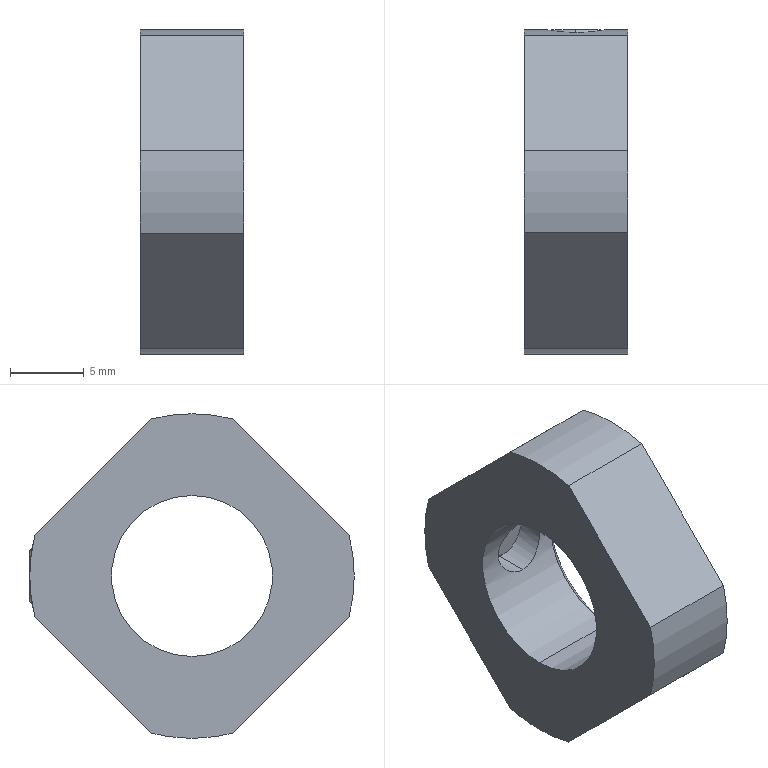Part | SolidWorks | features BaseBody 1 | 1 solid | 34 faces | box 6.99 x 22 x 22 mm | volume 1658 mm3 | plane 15 | cylinder 11 | cone 8 | commonest cylinder face diameters 22 x5 4 x4 10.918 x2
STEP:
#1=CARTESIAN_POINT('',(-0.49,-2.796,-10.639));
#2=VERTEX_POINT('',#1);
#3=CARTESIAN_POINT('',(-0.49,0.,-11.));
#4=VERTEX_POINT('',#3);
#5=CARTESIAN_POINT('',(-0.49,0.,0.));
#6=DIRECTION('',(1.,0.,0.));
#7=DIRECTION('',(0.,0.,-1.));
#8=AXIS2_PLACEMENT_3D('',#5,#6,#7);
#9=CIRCLE('',#8,11.);
#10=EDGE_CURVE('',#2,#4,#9,.T.);
#11=ORIENTED_EDGE('',*,*,#10,.T.);
#12=CARTESIAN_POINT('',(6.5,0.,-11.));
#13=VERTEX_POINT('',#12);
#14=CARTESIAN_POINT('',(-10.,0.,-11.));
#15=DIRECTION('',(1.,0.,0.));
#16=VECTOR('',#15,1000.);
#17=LINE('',#14,#16);
#18=EDGE_CURVE('',#4,#13,#17,.T.);
#19=ORIENTED_EDGE('',*,*,#18,.T.);
#20=CARTESIAN_POINT('',(6.5,-2.796,-10.639));
#21=VERTEX_POINT('',#20);
#22=CARTESIAN_POINT('',(6.5,0.,0.));
#23=DIRECTION('',(-1.,0.,0.));
#24=DIRECTION('',(0.,0.,-1.));
#25=AXIS2_PLACEMENT_3D('',#22,#23,#24);
#26=CIRCLE('',#25,11.);
#27=EDGE_CURVE('',#13,#21,#26,.T.);
#28=ORIENTED_EDGE('',*,*,#27,.T.);
#29=CARTESIAN_POINT('',(-13.5,-2.796,-10.639));
#30=DIRECTION('',(1.,0.,0.));
#31=VECTOR('',#30,1000.);
#32=LINE('',#29,#31);
#33=EDGE_CURVE('',#2,#21,#32,.T.);
#34=ORIENTED_EDGE('',*,*,#33,.F.);
#35=EDGE_LOOP('',(#11,#19,#28,#34));
#36=FACE_OUTER_BOUND('',#35,.T.);
#37=CARTESIAN_POINT('',(-10.,0.,0.));
#38=DIRECTION('',(1.,0.,0.));
#39=DIRECTION('',(0.,0.,-1.));
#40=AXIS2_PLACEMENT_3D('',#37,#38,#39);
#41=CYLINDRICAL_SURFACE('',#40,11.);
#42=ADVANCED_FACE('',(#36),#41,.T.);
#43=CARTESIAN_POINT('',(-0.49,0.,-5.459));
#44=VERTEX_POINT('',#43);
#45=CARTESIAN_POINT('',(-0.49,0.,5.459));
#46=VERTEX_POINT('',#45);
#47=CARTESIAN_POINT('',(-0.49,0.,0.));
#48=DIRECTION('',(-1.,0.,0.));
#49=DIRECTION('',(0.,0.,-1.));
#50=AXIS2_PLACEMENT_3D('',#47,#48,#49);
#51=CIRCLE('',#50,5.459);
#52=EDGE_CURVE('',#44,#46,#51,.T.);
#53=ORIENTED_EDGE('',*,*,#52,.T.);
#54=CARTESIAN_POINT('',(6.,0.,5.459));
#55=VERTEX_POINT('',#54);
#56=CARTESIAN_POINT('',(-10.,0.,5.459));
#57=DIRECTION('',(1.,0.,0.));
#58=VECTOR('',#57,1000.);
#59=LINE('',#56,#58);
#60=EDGE_CURVE('',#46,#55,#59,.T.);
#61=ORIENTED_EDGE('',*,*,#60,.T.);
#62=CARTESIAN_POINT('',(6.,0.,-5.459));
#63=VERTEX_POINT('',#62);
#64=CARTESIAN_POINT('',(6.,0.,0.));
#65=DIRECTION('',(-1.,0.,0.));
#66=DIRECTION('',(0.,0.,-1.));
#67=AXIS2_PLACEMENT_3D('',#64,#65,#66);
#68=CIRCLE('',#67,5.459);
#69=EDGE_CURVE('',#63,#55,#68,.T.);
#70=ORIENTED_EDGE('',*,*,#69,.F.);
#71=CARTESIAN_POINT('',(-10.,0.,-5.459));
#72=DIRECTION('',(1.,0.,0.));
#73=VECTOR('',#72,1000.);
#74=LINE('',#71,#73);
#75=EDGE_CURVE('',#44,#63,#74,.T.);
#76=ORIENTED_EDGE('',*,*,#75,.F.);
#77=EDGE_LOOP('',(#53,#61,#70,#76));
#78=FACE_OUTER_BOUND('',#77,.T.);
#79=CARTESIAN_POINT('',(-10.,0.,0.));
#80=DIRECTION('',(1.,0.,0.));
#81=DIRECTION('',(0.,0.,-1.));
#82=AXIS2_PLACEMENT_3D('',#79,#80,#81);
#83=CYLINDRICAL_SURFACE('',#82,5.459);
#84=ADVANCED_FACE('',(#78),#83,.F.);
#85=CARTESIAN_POINT('',(3.,10.7,-2.));
#86=VERTEX_POINT('',#85);
#87=CARTESIAN_POINT('',(3.,10.7,2.));
#88=VERTEX_POINT('',#87);
#89=CARTESIAN_POINT('',(3.,10.7,0.));
#90=DIRECTION('',(0.,1.,0.));
#91=DIRECTION('',(0.,0.,1.));
#92=AXIS2_PLACEMENT_3D('',#89,#90,#91);
#93=CIRCLE('',#92,2.);
#94=EDGE_CURVE('',#86,#88,#93,.T.);
#95=ORIENTED_EDGE('',*,*,#94,.F.);
#96=CARTESIAN_POINT('',(3.,10.817,-2.));
#97=VERTEX_POINT('',#96);
#98=CARTESIAN_POINT('',(3.,4.5,-2.));
#99=DIRECTION('',(0.,1.,0.));
#100=VECTOR('',#99,1000.);
#101=LINE('',#98,#100);
#102=EDGE_CURVE('',#86,#97,#101,.T.);
#103=ORIENTED_EDGE('',*,*,#102,.T.);
#104=CARTESIAN_POINT('',(3.,10.817,2.));
#105=VERTEX_POINT('',#104);
#106=CARTESIAN_POINT('',(3.,10.817,2.));
#107=CARTESIAN_POINT('',(2.737,10.817,2.));
#108=CARTESIAN_POINT('',(2.476,10.827,1.948));
#109=CARTESIAN_POINT('',(2.112,10.852,1.797));
#110=CARTESIAN_POINT('',(1.997,10.863,1.735));
#111=CARTESIAN_POINT('',(1.78,10.885,1.59));
#112=CARTESIAN_POINT('',(1.678,10.897,1.506));
#113=CARTESIAN_POINT('',(1.493,10.921,1.322));
#114=CARTESIAN_POINT('',(1.411,10.933,1.221));
#115=CARTESIAN_POINT('',(1.265,10.955,1.004));
#116=CARTESIAN_POINT('',(1.203,10.965,0.8867));
#117=CARTESIAN_POINT('',(1.053,10.99,0.5258));
#118=CARTESIAN_POINT('',(0.9999,11.,0.2626));
#119=CARTESIAN_POINT('',(1.,11.,-0.2643));
#120=CARTESIAN_POINT('',(1.052,10.99,-0.524));
#121=CARTESIAN_POINT('',(1.204,10.965,-0.8894));
#122=CARTESIAN_POINT('',(1.265,10.955,-1.004));
#123=CARTESIAN_POINT('',(1.41,10.933,-1.221));
#124=CARTESIAN_POINT('',(1.494,10.921,-1.323));
#125=CARTESIAN_POINT('',(1.679,10.897,-1.508));
#126=CARTESIAN_POINT('',(1.78,10.885,-1.59));
#127=CARTESIAN_POINT('',(1.997,10.863,-1.735));
#128=CARTESIAN_POINT('',(2.114,10.852,-1.798));
#129=CARTESIAN_POINT('',(2.475,10.827,-1.947));
#130=CARTESIAN_POINT('',(2.739,10.817,-2.));
#131=CARTESIAN_POINT('',(3.,10.817,-2.));
#132=B_SPLINE_CURVE_WITH_KNOTS('',3,(#106,#107,#108,#109,#110,#111,#112,#113,#114,#115,#116,#117,#118,#119,#120,#121,#122,#123,#124,#125,#126,#127,#128,#129,#130,#131),.UNSPECIFIED.,.F.,.F.,(4,2,2,2,2,2,2,2,2,2,2,2,4),(0.009301,0.01008,0.01048,0.01087,0.01126,0.01165,0.01243,0.01322,0.01361,0.014,0.01439,0.01478,0.01557),.UNSPECIFIED.);
#133=EDGE_CURVE('',#105,#97,#132,.T.);
#134=ORIENTED_EDGE('',*,*,#133,.F.);
#135=CARTESIAN_POINT('',(3.,4.5,2.));
#136=DIRECTION('',(0.,1.,0.));
#137=VECTOR('',#136,1000.);
#138=LINE('',#135,#137);
#139=EDGE_CURVE('',#88,#105,#138,.T.);
#140=ORIENTED_EDGE('',*,*,#139,.F.);
#141=EDGE_LOOP('',(#95,#103,#134,#140));
#142=FACE_OUTER_BOUND('',#141,.T.);
#143=CARTESIAN_POINT('',(3.,4.5,0.));
#144=DIRECTION('',(0.,1.,0.));
#145=DIRECTION('',(0.,0.,1.));
#146=AXIS2_PLACEMENT_3D('',#143,#144,#145);
#147=CYLINDRICAL_SURFACE('',#146,2.);
#148=ADVANCED_FACE('',(#142),#147,.F.);
#149=CARTESIAN_POINT('',(3.,5.079,2.));
#150=VERTEX_POINT('',#149);
#151=CARTESIAN_POINT('',(3.,5.079,-2.));
#152=VERTEX_POINT('',#151);
#153=CARTESIAN_POINT('',(3.,5.079,2.));
#154=CARTESIAN_POINT('',(2.737,5.079,2.));
#155=CARTESIAN_POINT('',(2.472,5.101,1.947));
#156=CARTESIAN_POINT('',(2.111,5.155,1.796));
#157=CARTESIAN_POINT('',(1.994,5.177,1.733));
#158=CARTESIAN_POINT('',(1.778,5.223,1.588));
#159=CARTESIAN_POINT('',(1.678,5.248,1.506));
#160=CARTESIAN_POINT('',(1.494,5.297,1.323));
#161=CARTESIAN_POINT('',(1.411,5.322,1.221));
#162=CARTESIAN_POINT('',(1.266,5.367,1.006));
#163=CARTESIAN_POINT('',(1.205,5.387,0.8911));
#164=CARTESIAN_POINT('',(1.052,5.439,0.526));
#165=CARTESIAN_POINT('',(0.9999,5.459,0.2647));
#166=CARTESIAN_POINT('',(1.,5.459,-0.1332));
#167=CARTESIAN_POINT('',(1.013,5.454,-0.264));
#168=CARTESIAN_POINT('',(1.065,5.436,-0.522));
#169=CARTESIAN_POINT('',(1.104,5.422,-0.6499));
#170=CARTESIAN_POINT('',(1.255,5.37,-1.012));
#171=CARTESIAN_POINT('',(1.404,5.321,-1.233));
#172=CARTESIAN_POINT('',(1.678,5.248,-1.507));
#173=CARTESIAN_POINT('',(1.78,5.223,-1.59));
#174=CARTESIAN_POINT('',(1.997,5.177,-1.735));
#175=CARTESIAN_POINT('',(2.111,5.155,-1.796));
#176=CARTESIAN_POINT('',(2.352,5.119,-1.897));
#177=CARTESIAN_POINT('',(2.48,5.104,-1.936));
#178=CARTESIAN_POINT('',(2.737,5.085,-1.987));
#179=CARTESIAN_POINT('',(2.868,5.079,-2.));
#180=CARTESIAN_POINT('',(3.,5.079,-2.));
#181=B_SPLINE_CURVE_WITH_KNOTS('',3,(#153,#154,#155,#156,#157,#158,#159,#160,#161,#162,#163,#164,#165,#166,#167,#168,#169,#170,#171,#172,#173,#174,#175,#176,#177,#178,#179,#180),.UNSPECIFIED.,.F.,.F.,(4,2,2,2,2,2,2,2,2,2,2,2,2,4),(0.006208,0.006997,0.007391,0.007785,0.008179,0.008573,0.009362,0.009756,0.01015,0.01094,0.01133,0.01173,0.01212,0.01252),.UNSPECIFIED.);
#182=EDGE_CURVE('',#150,#152,#181,.T.);
#183=ORIENTED_EDGE('',*,*,#182,.T.);
#184=CARTESIAN_POINT('',(3.,7.3,-2.));
#185=VERTEX_POINT('',#184);
#186=CARTESIAN_POINT('',(3.,4.5,-2.));
#187=DIRECTION('',(0.,1.,0.));
#188=VECTOR('',#187,1000.);
#189=LINE('',#186,#188);
#190=EDGE_CURVE('',#152,#185,#189,.T.);
#191=ORIENTED_EDGE('',*,*,#190,.T.);
#192=CARTESIAN_POINT('',(3.,7.3,2.));
#193=VERTEX_POINT('',#192);
#194=CARTESIAN_POINT('',(3.,7.3,0.));
#195=DIRECTION('',(0.,-1.,0.));
#196=DIRECTION('',(0.,0.,1.));
#197=AXIS2_PLACEMENT_3D('',#194,#195,#196);
#198=CIRCLE('',#197,2.);
#199=EDGE_CURVE('',#193,#185,#198,.T.);
#200=ORIENTED_EDGE('',*,*,#199,.F.);
#201=CARTESIAN_POINT('',(3.,4.5,2.));
#202=DIRECTION('',(0.,1.,0.));
#203=VECTOR('',#202,1000.);
#204=LINE('',#201,#203);
#205=EDGE_CURVE('',#150,#193,#204,.T.);
#206=ORIENTED_EDGE('',*,*,#205,.F.);
#207=EDGE_LOOP('',(#183,#191,#200,#206));
#208=FACE_OUTER_BOUND('',#207,.T.);
#209=CARTESIAN_POINT('',(3.,4.5,0.));
#210=DIRECTION('',(0.,1.,0.));
#211=DIRECTION('',(0.,0.,1.));
#212=AXIS2_PLACEMENT_3D('',#209,#210,#211);
#213=CYLINDRICAL_SURFACE('',#212,2.);
#214=ADVANCED_FACE('',(#208),#213,.F.);
#215=ORIENTED_EDGE('',*,*,#69,.T.);
#216=CARTESIAN_POINT('',(6.5,0.,5.959));
#217=VERTEX_POINT('',#216);
#218=CARTESIAN_POINT('',(6.5,0.,5.959));
#219=DIRECTION('',(0.7071,0.,0.7071));
#220=VECTOR('',#219,1000.);
#221=LINE('',#218,#220);
#222=EDGE_CURVE('',#55,#217,#221,.T.);
#223=ORIENTED_EDGE('',*,*,#222,.T.);
#224=CARTESIAN_POINT('',(6.5,0.,-5.959));
#225=VERTEX_POINT('',#224);
#226=CARTESIAN_POINT('',(6.5,0.,0.));
#227=DIRECTION('',(-1.,0.,0.));
#228=DIRECTION('',(0.,0.,-1.));
#229=AXIS2_PLACEMENT_3D('',#226,#227,#228);
#230=CIRCLE('',#229,5.959);
#231=EDGE_CURVE('',#225,#217,#230,.T.);
#232=ORIENTED_EDGE('',*,*,#231,.F.);
#233=CARTESIAN_POINT('',(6.5,0.,-5.959));
#234=DIRECTION('',(0.7071,0.,-0.7071));
#235=VECTOR('',#234,1000.);
#236=LINE('',#233,#235);
#237=EDGE_CURVE('',#63,#225,#236,.T.);
#238=ORIENTED_EDGE('',*,*,#237,.F.);
#239=EDGE_LOOP('',(#215,#223,#232,#238));
#240=FACE_OUTER_BOUND('',#239,.T.);
#241=CARTESIAN_POINT('',(6.5,0.,0.));
#242=DIRECTION('',(1.,0.,0.));
#243=DIRECTION('',(0.,0.,-1.));
#244=AXIS2_PLACEMENT_3D('',#241,#242,#243);
#245=CONICAL_SURFACE('',#244,5.959,0.7854);
#246=ADVANCED_FACE('',(#240),#245,.F.);
#247=CARTESIAN_POINT('',(3.,11.,-1.7));
#248=VERTEX_POINT('',#247);
#249=CARTESIAN_POINT('',(3.,11.,1.7));
#250=VERTEX_POINT('',#249);
#251=CARTESIAN_POINT('',(3.,11.,0.));
#252=DIRECTION('',(0.,-1.,0.));
#253=DIRECTION('',(0.,0.,-1.));
#254=AXIS2_PLACEMENT_3D('',#251,#252,#253);
#255=CIRCLE('',#254,1.7);
#256=EDGE_CURVE('',#248,#250,#255,.T.);
#257=ORIENTED_EDGE('',*,*,#256,.T.);
#258=CARTESIAN_POINT('',(3.,10.7,2.));
#259=DIRECTION('',(0.,-0.7071,0.7071));
#260=VECTOR('',#259,1000.);
#261=LINE('',#258,#260);
#262=EDGE_CURVE('',#250,#88,#261,.T.);
#263=ORIENTED_EDGE('',*,*,#262,.T.);
#264=CARTESIAN_POINT('',(3.,10.7,0.));
#265=DIRECTION('',(0.,1.,0.));
#266=DIRECTION('',(0.,0.,1.));
#267=AXIS2_PLACEMENT_3D('',#264,#265,#266);
#268=CIRCLE('',#267,2.);
#269=EDGE_CURVE('',#88,#86,#268,.T.);
#270=ORIENTED_EDGE('',*,*,#269,.T.);
#271=CARTESIAN_POINT('',(3.,10.7,-2.));
#272=DIRECTION('',(0.,-0.7071,-0.7071));
#273=VECTOR('',#272,1000.);
#274=LINE('',#271,#273);
#275=EDGE_CURVE('',#248,#86,#274,.T.);
#276=ORIENTED_EDGE('',*,*,#275,.F.);
#277=EDGE_LOOP('',(#257,#263,#270,#276));
#278=FACE_OUTER_BOUND('',#277,.T.);
#279=CARTESIAN_POINT('',(3.,10.7,0.));
#280=DIRECTION('',(0.,-1.,0.));
#281=DIRECTION('',(0.,0.,-1.));
#282=AXIS2_PLACEMENT_3D('',#279,#280,#281);
#283=CONICAL_SURFACE('',#282,2.,0.7854);
#284=ADVANCED_FACE('',(#278),#283,.T.);
#285=CARTESIAN_POINT('',(3.,7.,1.7));
#286=VERTEX_POINT('',#285);
#287=CARTESIAN_POINT('',(3.,7.,-1.7));
#288=VERTEX_POINT('',#287);
#289=CARTESIAN_POINT('',(3.,7.,0.));
#290=DIRECTION('',(0.,1.,0.));
#291=DIRECTION('',(0.,0.,1.));
#292=AXIS2_PLACEMENT_3D('',#289,#290,#291);
#293=CIRCLE('',#292,1.7);
#294=EDGE_CURVE('',#286,#288,#293,.T.);
#295=ORIENTED_EDGE('',*,*,#294,.T.);
#296=CARTESIAN_POINT('',(3.,7.3,-2.));
#297=DIRECTION('',(0.,0.7071,-0.7071));
#298=VECTOR('',#297,1000.);
#299=LINE('',#296,#298);
#300=EDGE_CURVE('',#288,#185,#299,.T.);
#301=ORIENTED_EDGE('',*,*,#300,.T.);
#302=CARTESIAN_POINT('',(3.,7.3,0.));
#303=DIRECTION('',(0.,-1.,0.));
#304=DIRECTION('',(0.,0.,1.));
#305=AXIS2_PLACEMENT_3D('',#302,#303,#304);
#306=CIRCLE('',#305,2.);
#307=EDGE_CURVE('',#185,#193,#306,.T.);
#308=ORIENTED_EDGE('',*,*,#307,.T.);
#309=CARTESIAN_POINT('',(3.,7.3,2.));
#310=DIRECTION('',(0.,0.7071,0.7071));
#311=VECTOR('',#310,1000.);
#312=LINE('',#309,#311);
#313=EDGE_CURVE('',#286,#193,#312,.T.);
#314=ORIENTED_EDGE('',*,*,#313,.F.);
#315=EDGE_LOOP('',(#295,#301,#308,#314));
#316=FACE_OUTER_BOUND('',#315,.T.);
#317=CARTESIAN_POINT('',(3.,7.3,0.));
#318=DIRECTION('',(0.,1.,0.));
#319=DIRECTION('',(0.,0.,1.));
#320=AXIS2_PLACEMENT_3D('',#317,#318,#319);
#321=CONICAL_SURFACE('',#320,2.,0.7854);
#322=ADVANCED_FACE('',(#316),#321,.T.);
#323=CARTESIAN_POINT('',(2.01,10.995,-0.5716));
#324=VERTEX_POINT('',#323);
#325=CARTESIAN_POINT('',(3.,10.995,-1.143));
#326=VERTEX_POINT('',#325);
#327=CARTESIAN_POINT('',(2.01,10.995,-0.5716));
#328=CARTESIAN_POINT('',(2.17,10.931,-0.6638));
#329=CARTESIAN_POINT('',(2.337,10.888,-0.7603));
#330=CARTESIAN_POINT('',(2.673,10.888,-0.9544));
#331=CARTESIAN_POINT('',(2.84,10.931,-1.051));
#332=CARTESIAN_POINT('',(3.,10.995,-1.143));
#333=B_SPLINE_CURVE_WITH_KNOTS('',3,(#327,#328,#329,#330,#331,#332),.UNSPECIFIED.,.F.,.F.,(4,2,4),(-0.0007691,-0.0001856,0.0003979),.UNSPECIFIED.);
#334=EDGE_CURVE('',#324,#326,#333,.T.);
#335=ORIENTED_EDGE('',*,*,#334,.T.);
#336=CARTESIAN_POINT('',(3.,11.,-1.15));
#337=VERTEX_POINT('',#336);
#338=CARTESIAN_POINT('',(3.,11.,-1.15));
#339=DIRECTION('',(0.,0.5736,-0.8192));
#340=VECTOR('',#339,1000.);
#341=LINE('',#338,#340);
#342=EDGE_CURVE('',#326,#337,#341,.T.);
#343=ORIENTED_EDGE('',*,*,#342,.T.);
#344=CARTESIAN_POINT('',(3.,11.,1.15));
#345=VERTEX_POINT('',#344);
#346=CARTESIAN_POINT('',(3.,11.,0.));
#347=DIRECTION('',(0.,1.,0.));
#348=DIRECTION('',(0.,0.,1.));
#349=AXIS2_PLACEMENT_3D('',#346,#347,#348);
#350=CIRCLE('',#349,1.15);
#351=EDGE_CURVE('',#337,#345,#350,.T.);
#352=ORIENTED_EDGE('',*,*,#351,.T.);
#353=CARTESIAN_POINT('',(3.,10.995,1.143));
#354=VERTEX_POINT('',#353);
#355=CARTESIAN_POINT('',(3.,11.,1.15));
#356=DIRECTION('',(0.,0.5736,0.8192));
#357=VECTOR('',#356,1000.);
#358=LINE('',#355,#357);
#359=EDGE_CURVE('',#354,#345,#358,.T.);
#360=ORIENTED_EDGE('',*,*,#359,.F.);
#361=CARTESIAN_POINT('',(2.01,10.995,0.5716));
#362=VERTEX_POINT('',#361);
#363=CARTESIAN_POINT('',(2.01,10.995,0.5716));
#364=CARTESIAN_POINT('',(2.17,10.931,0.6638));
#365=CARTESIAN_POINT('',(2.337,10.888,0.7603));
#366=CARTESIAN_POINT('',(2.673,10.888,0.9544));
#367=CARTESIAN_POINT('',(2.84,10.931,1.051));
#368=CARTESIAN_POINT('',(3.,10.995,1.143));
#369=B_SPLINE_CURVE_WITH_KNOTS('',3,(#363,#364,#365,#366,#367,#368),.UNSPECIFIED.,.F.,.F.,(4,2,4),(0.,0.0005835,0.001167),.UNSPECIFIED.);
#370=EDGE_CURVE('',#362,#354,#369,.T.);
#371=ORIENTED_EDGE('',*,*,#370,.F.);
#372=CARTESIAN_POINT('',(2.01,10.995,0.5716));
#373=CARTESIAN_POINT('',(2.01,10.931,0.3872));
#374=CARTESIAN_POINT('',(2.01,10.888,0.1941));
#375=CARTESIAN_POINT('',(2.01,10.888,-0.1941));
#376=CARTESIAN_POINT('',(2.01,10.931,-0.3872));
#377=CARTESIAN_POINT('',(2.01,10.995,-0.5716));
#378=B_SPLINE_CURVE_WITH_KNOTS('',3,(#372,#373,#374,#375,#376,#377),.UNSPECIFIED.,.F.,.F.,(4,2,4),(-0.0007691,-0.0001856,0.0003979),.UNSPECIFIED.);
#379=EDGE_CURVE('',#362,#324,#378,.T.);
#380=ORIENTED_EDGE('',*,*,#379,.T.);
#381=EDGE_LOOP('',(#335,#343,#352,#360,#371,#380));
#382=FACE_OUTER_BOUND('',#381,.T.);
#383=CARTESIAN_POINT('',(3.,11.,0.));
#384=DIRECTION('',(0.,1.,0.));
#385=DIRECTION('',(0.,0.,1.));
#386=AXIS2_PLACEMENT_3D('',#383,#384,#385);
#387=CONICAL_SURFACE('',#386,1.15,0.9599);
#388=ADVANCED_FACE('',(#382),#387,.F.);
#389=CARTESIAN_POINT('',(-0.49,-10.639,2.796));
#390=VERTEX_POINT('',#389);
#391=CARTESIAN_POINT('',(-0.49,-10.639,-2.796));
#392=VERTEX_POINT('',#391);
#393=CARTESIAN_POINT('',(-0.49,0.,0.));
#394=DIRECTION('',(1.,0.,0.));
#395=DIRECTION('',(0.,0.,-1.));
#396=AXIS2_PLACEMENT_3D('',#393,#394,#395);
#397=CIRCLE('',#396,11.);
#398=EDGE_CURVE('',#390,#392,#397,.T.);
#399=ORIENTED_EDGE('',*,*,#398,.F.);
#400=CARTESIAN_POINT('',(-0.49,-2.796,10.639));
#401=VERTEX_POINT('',#400);
#402=CARTESIAN_POINT('',(-0.49,-2.796,10.639));
#403=DIRECTION('',(0.,-0.7071,-0.7071));
#404=VECTOR('',#403,1000.);
#405=LINE('',#402,#404);
#406=EDGE_CURVE('',#401,#390,#405,.T.);
#407=ORIENTED_EDGE('',*,*,#406,.F.);
#408=CARTESIAN_POINT('',(-0.49,2.796,10.639));
#409=VERTEX_POINT('',#408);
#410=CARTESIAN_POINT('',(-0.49,0.,0.));
#411=DIRECTION('',(1.,0.,0.));
#412=DIRECTION('',(0.,0.,-1.));
#413=AXIS2_PLACEMENT_3D('',#410,#411,#412);
#414=CIRCLE('',#413,11.);
#415=EDGE_CURVE('',#409,#401,#414,.T.);
#416=ORIENTED_EDGE('',*,*,#415,.F.);
#417=CARTESIAN_POINT('',(-0.49,10.639,2.796));
#418=VERTEX_POINT('',#417);
#419=CARTESIAN_POINT('',(-0.49,10.639,2.796));
#420=DIRECTION('',(0.,-0.7071,0.7071));
#421=VECTOR('',#420,1000.);
#422=LINE('',#419,#421);
#423=EDGE_CURVE('',#418,#409,#422,.T.);
#424=ORIENTED_EDGE('',*,*,#423,.F.);
#425=CARTESIAN_POINT('',(-0.49,10.639,-2.796));
#426=VERTEX_POINT('',#425);
#427=CARTESIAN_POINT('',(-0.49,0.,0.));
#428=DIRECTION('',(1.,0.,0.));
#429=DIRECTION('',(0.,0.,-1.));
#430=AXIS2_PLACEMENT_3D('',#427,#428,#429);
#431=CIRCLE('',#430,11.);
#432=EDGE_CURVE('',#426,#418,#431,.T.);
#433=ORIENTED_EDGE('',*,*,#432,.F.);
#434=CARTESIAN_POINT('',(-0.49,2.796,-10.639));
#435=VERTEX_POINT('',#434);
#436=CARTESIAN_POINT('',(-0.49,2.796,-10.639));
#437=DIRECTION('',(0.,0.7071,0.7071));
#438=VECTOR('',#437,1000.);
#439=LINE('',#436,#438);
#440=EDGE_CURVE('',#435,#426,#439,.T.);
#441=ORIENTED_EDGE('',*,*,#440,.F.);
#442=CARTESIAN_POINT('',(-0.49,0.,0.));
#443=DIRECTION('',(1.,0.,0.));
#444=DIRECTION('',(0.,0.,-1.));
#445=AXIS2_PLACEMENT_3D('',#442,#443,#444);
#446=CIRCLE('',#445,11.);
#447=EDGE_CURVE('',#4,#435,#446,.T.);
#448=ORIENTED_EDGE('',*,*,#447,.F.);
#449=ORIENTED_EDGE('',*,*,#10,.F.);
#450=CARTESIAN_POINT('',(-0.49,-10.639,-2.796));
#451=DIRECTION('',(0.,0.7071,-0.7071));
#452=VECTOR('',#451,1000.);
#453=LINE('',#450,#452);
#454=EDGE_CURVE('',#392,#2,#453,.T.);
#455=ORIENTED_EDGE('',*,*,#454,.F.);
#456=EDGE_LOOP('',(#399,#407,#416,#424,#433,#441,#448,#449,#455));
#457=FACE_OUTER_BOUND('',#456,.T.);
#458=ORIENTED_EDGE('',*,*,#52,.F.);
#459=CARTESIAN_POINT('',(-0.49,0.,0.));
#460=DIRECTION('',(-1.,0.,0.));
#461=DIRECTION('',(0.,0.,-1.));
#462=AXIS2_PLACEMENT_3D('',#459,#460,#461);
#463=CIRCLE('',#462,5.459);
#464=EDGE_CURVE('',#46,#44,#463,.T.);
#465=ORIENTED_EDGE('',*,*,#464,.F.);
#466=EDGE_LOOP('',(#458,#465));
#467=FACE_BOUND('',#466,.T.);
#468=CARTESIAN_POINT('',(-0.49,0.,0.));
#469=DIRECTION('',(1.,0.,0.));
#470=DIRECTION('',(0.,0.,-1.));
#471=AXIS2_PLACEMENT_3D('',#468,#469,#470);
#472=PLANE('',#471);
#473=ADVANCED_FACE('',(#457,#467),#472,.F.);
#474=CARTESIAN_POINT('',(6.5,-10.639,-2.796));
#475=VERTEX_POINT('',#474);
#476=CARTESIAN_POINT('',(6.5,-13.435,0.));
#477=DIRECTION('',(0.,-0.7071,0.7071));
#478=VECTOR('',#477,1000.);
#479=LINE('',#476,#478);
#480=EDGE_CURVE('',#21,#475,#479,.T.);
#481=ORIENTED_EDGE('',*,*,#480,.T.);
#482=CARTESIAN_POINT('',(-13.5,-10.639,-2.796));
#483=DIRECTION('',(-1.,0.,0.));
#484=VECTOR('',#483,1000.);
#485=LINE('',#482,#484);
#486=EDGE_CURVE('',#475,#392,#485,.T.);
#487=ORIENTED_EDGE('',*,*,#486,.T.);
#488=ORIENTED_EDGE('',*,*,#454,.T.);
#489=ORIENTED_EDGE('',*,*,#33,.T.);
#490=EDGE_LOOP('',(#481,#487,#488,#489));
#491=FACE_OUTER_BOUND('',#490,.T.);
#492=CARTESIAN_POINT('',(-13.5,-13.435,0.));
#493=DIRECTION('',(0.,-0.7071,-0.7071));
#494=DIRECTION('',(0.,0.7071,-0.7071));
#495=AXIS2_PLACEMENT_3D('',#492,#493,#494);
#496=PLANE('',#495);
#497=ADVANCED_FACE('',(#491),#496,.T.);
#498=ORIENTED_EDGE('',*,*,#486,.F.);
#499=CARTESIAN_POINT('',(6.5,-10.639,2.796));
#500=VERTEX_POINT('',#499);
#501=CARTESIAN_POINT('',(6.5,0.,0.));
#502=DIRECTION('',(-1.,0.,0.));
#503=DIRECTION('',(0.,0.,-1.));
#504=AXIS2_PLACEMENT_3D('',#501,#502,#503);
#505=CIRCLE('',#504,11.);
#506=EDGE_CURVE('',#475,#500,#505,.T.);
#507=ORIENTED_EDGE('',*,*,#506,.T.);
#508=CARTESIAN_POINT('',(-10.,-10.639,2.796));
#509=DIRECTION('',(-1.,0.,0.));
#510=VECTOR('',#509,1000.);
#511=LINE('',#508,#510);
#512=EDGE_CURVE('',#500,#390,#511,.T.);
#513=ORIENTED_EDGE('',*,*,#512,.T.);
#514=ORIENTED_EDGE('',*,*,#398,.T.);
#515=EDGE_LOOP('',(#498,#507,#513,#514));
#516=FACE_OUTER_BOUND('',#515,.T.);
#517=CARTESIAN_POINT('',(-10.,0.,0.));
#518=DIRECTION('',(1.,0.,0.));
#519=DIRECTION('',(0.,0.,-1.));
#520=AXIS2_PLACEMENT_3D('',#517,#518,#519);
#521=CYLINDRICAL_SURFACE('',#520,11.);
#522=ADVANCED_FACE('',(#516),#521,.T.);
#523=CARTESIAN_POINT('',(6.5,-2.796,10.639));
#524=VERTEX_POINT('',#523);
#525=CARTESIAN_POINT('',(6.5,0.,13.435));
#526=DIRECTION('',(0.,0.7071,0.7071));
#527=VECTOR('',#526,1000.);
#528=LINE('',#525,#527);
#529=EDGE_CURVE('',#500,#524,#528,.T.);
#530=ORIENTED_EDGE('',*,*,#529,.T.);
#531=CARTESIAN_POINT('',(-13.5,-2.796,10.639));
#532=DIRECTION('',(-1.,0.,0.));
#533=VECTOR('',#532,1000.);
#534=LINE('',#531,#533);
#535=EDGE_CURVE('',#524,#401,#534,.T.);
#536=ORIENTED_EDGE('',*,*,#535,.T.);
#537=ORIENTED_EDGE('',*,*,#406,.T.);
#538=ORIENTED_EDGE('',*,*,#512,.F.);
#539=EDGE_LOOP('',(#530,#536,#537,#538));
#540=FACE_OUTER_BOUND('',#539,.T.);
#541=CARTESIAN_POINT('',(-13.5,0.,13.435));
#542=DIRECTION('',(0.,-0.7071,0.7071));
#543=DIRECTION('',(0.,-0.7071,-0.7071));
#544=AXIS2_PLACEMENT_3D('',#541,#542,#543);
#545=PLANE('',#544);
#546=ADVANCED_FACE('',(#540),#545,.T.);
#547=CARTESIAN_POINT('',(6.5,2.796,10.639));
#548=VERTEX_POINT('',#547);
#549=CARTESIAN_POINT('',(6.5,0.,0.));
#550=DIRECTION('',(-1.,0.,0.));
#551=DIRECTION('',(0.,0.,-1.));
#552=AXIS2_PLACEMENT_3D('',#549,#550,#551);
#553=CIRCLE('',#552,11.);
#554=EDGE_CURVE('',#524,#548,#553,.T.);
#555=ORIENTED_EDGE('',*,*,#554,.T.);
#556=CARTESIAN_POINT('',(-10.,2.796,10.639));
#557=DIRECTION('',(-1.,0.,0.));
#558=VECTOR('',#557,1000.);
#559=LINE('',#556,#558);
#560=EDGE_CURVE('',#548,#409,#559,.T.);
#561=ORIENTED_EDGE('',*,*,#560,.T.);
#562=ORIENTED_EDGE('',*,*,#415,.T.);
#563=ORIENTED_EDGE('',*,*,#535,.F.);
#564=EDGE_LOOP('',(#555,#561,#562,#563));
#565=FACE_OUTER_BOUND('',#564,.T.);
#566=CARTESIAN_POINT('',(-10.,0.,0.));
#567=DIRECTION('',(1.,0.,0.));
#568=DIRECTION('',(0.,0.,-1.));
#569=AXIS2_PLACEMENT_3D('',#566,#567,#568);
#570=CYLINDRICAL_SURFACE('',#569,11.);
#571=ADVANCED_FACE('',(#565),#570,.T.);
#572=CARTESIAN_POINT('',(6.5,10.639,2.796));
#573=VERTEX_POINT('',#572);
#574=CARTESIAN_POINT('',(6.5,13.435,0.));
#575=DIRECTION('',(0.,0.7071,-0.7071));
#576=VECTOR('',#575,1000.);
#577=LINE('',#574,#576);
#578=EDGE_CURVE('',#548,#573,#577,.T.);
#579=ORIENTED_EDGE('',*,*,#578,.T.);
#580=CARTESIAN_POINT('',(-13.5,10.639,2.796));
#581=DIRECTION('',(-1.,0.,0.));
#582=VECTOR('',#581,1000.);
#583=LINE('',#580,#582);
#584=EDGE_CURVE('',#573,#418,#583,.T.);
#585=ORIENTED_EDGE('',*,*,#584,.T.);
#586=ORIENTED_EDGE('',*,*,#423,.T.);
#587=ORIENTED_EDGE('',*,*,#560,.F.);
#588=EDGE_LOOP('',(#579,#585,#586,#587));
#589=FACE_OUTER_BOUND('',#588,.T.);
#590=CARTESIAN_POINT('',(-13.5,13.435,0.));
#591=DIRECTION('',(0.,0.7071,0.7071));
#592=DIRECTION('',(0.,-0.7071,0.7071));
#593=AXIS2_PLACEMENT_3D('',#590,#591,#592);
#594=PLANE('',#593);
#595=ADVANCED_FACE('',(#589),#594,.T.);
#596=ORIENTED_EDGE('',*,*,#133,.T.);
#597=CARTESIAN_POINT('',(3.,10.817,-2.));
#598=CARTESIAN_POINT('',(3.131,10.817,-2.));
#599=CARTESIAN_POINT('',(3.262,10.819,-1.987));
#600=CARTESIAN_POINT('',(3.521,10.828,-1.936));
#601=CARTESIAN_POINT('',(3.645,10.835,-1.898));
#602=CARTESIAN_POINT('',(3.887,10.852,-1.797));
#603=CARTESIAN_POINT('',(4.004,10.863,-1.735));
#604=CARTESIAN_POINT('',(4.221,10.885,-1.59));
#605=CARTESIAN_POINT('',(4.321,10.897,-1.507));
#606=CARTESIAN_POINT('',(4.6,10.933,-1.229));
#607=CARTESIAN_POINT('',(4.747,10.956,-1.009));
#608=CARTESIAN_POINT('',(4.898,10.982,-0.644));
#609=CARTESIAN_POINT('',(4.936,10.988,-0.519));
#610=CARTESIAN_POINT('',(4.987,10.998,-0.263));
#611=CARTESIAN_POINT('',(5.,11.,-0.1303));
#612=CARTESIAN_POINT('',(5.,11.,0.1321));
#613=CARTESIAN_POINT('',(4.987,10.998,0.262));
#614=CARTESIAN_POINT('',(4.936,10.988,0.5192));
#615=CARTESIAN_POINT('',(4.897,10.982,0.6466));
#616=CARTESIAN_POINT('',(4.747,10.956,1.008));
#617=CARTESIAN_POINT('',(4.598,10.933,1.231));
#618=CARTESIAN_POINT('',(4.322,10.897,1.506));
#619=CARTESIAN_POINT('',(4.22,10.885,1.59));
#620=CARTESIAN_POINT('',(4.002,10.862,1.736));
#621=CARTESIAN_POINT('',(3.887,10.852,1.797));
#622=CARTESIAN_POINT('',(3.646,10.835,1.897));
#623=CARTESIAN_POINT('',(3.518,10.828,1.936));
#624=CARTESIAN_POINT('',(3.262,10.819,1.987));
#625=CARTESIAN_POINT('',(3.132,10.817,2.));
#626=CARTESIAN_POINT('',(3.,10.817,2.));
#627=B_SPLINE_CURVE_WITH_KNOTS('',3,(#597,#598,#599,#600,#601,#602,#603,#604,#605,#606,#607,#608,#609,#610,#611,#612,#613,#614,#615,#616,#617,#618,#619,#620,#621,#622,#623,#624,#625,#626),.UNSPECIFIED.,.F.,.F.,(4,2,2,2,2,2,2,2,2,2,2,2,2,2,4),(0.003035,0.003427,0.003818,0.00421,0.004602,0.005385,0.005777,0.006168,0.00656,0.006952,0.007735,0.008126,0.008518,0.00891,0.009301),.UNSPECIFIED.);
#628=EDGE_CURVE('',#97,#105,#627,.T.);
#629=ORIENTED_EDGE('',*,*,#628,.T.);
#630=EDGE_LOOP('',(#596,#629));
#631=FACE_BOUND('',#630,.T.);
#632=CARTESIAN_POINT('',(6.5,10.639,-2.796));
#633=VERTEX_POINT('',#632);
#634=CARTESIAN_POINT('',(6.5,0.,0.));
#635=DIRECTION('',(-1.,0.,0.));
#636=DIRECTION('',(0.,0.,-1.));
#637=AXIS2_PLACEMENT_3D('',#634,#635,#636);
#638=CIRCLE('',#637,11.);
#639=EDGE_CURVE('',#573,#633,#638,.T.);
#640=ORIENTED_EDGE('',*,*,#639,.T.);
#641=CARTESIAN_POINT('',(-10.,10.639,-2.796));
#642=DIRECTION('',(-1.,0.,0.));
#643=VECTOR('',#642,1000.);
#644=LINE('',#641,#643);
#645=EDGE_CURVE('',#633,#426,#644,.T.);
#646=ORIENTED_EDGE('',*,*,#645,.T.);
#647=ORIENTED_EDGE('',*,*,#432,.T.);
#648=ORIENTED_EDGE('',*,*,#584,.F.);
#649=EDGE_LOOP('',(#640,#646,#647,#648));
#650=FACE_OUTER_BOUND('',#649,.T.);
#651=CARTESIAN_POINT('',(-10.,0.,0.));
#652=DIRECTION('',(1.,0.,0.));
#653=DIRECTION('',(0.,0.,-1.));
#654=AXIS2_PLACEMENT_3D('',#651,#652,#653);
#655=CYLINDRICAL_SURFACE('',#654,11.);
#656=ADVANCED_FACE('',(#631,#650),#655,.T.);
#657=CARTESIAN_POINT('',(6.5,2.796,-10.639));
#658=VERTEX_POINT('',#657);
#659=CARTESIAN_POINT('',(6.5,0.,-13.435));
#660=DIRECTION('',(0.,-0.7071,-0.7071));
#661=VECTOR('',#660,1000.);
#662=LINE('',#659,#661);
#663=EDGE_CURVE('',#633,#658,#662,.T.);
#664=ORIENTED_EDGE('',*,*,#663,.T.);
#665=CARTESIAN_POINT('',(-13.5,2.796,-10.639));
#666=DIRECTION('',(-1.,0.,0.));
#667=VECTOR('',#666,1000.);
#668=LINE('',#665,#667);
#669=EDGE_CURVE('',#658,#435,#668,.T.);
#670=ORIENTED_EDGE('',*,*,#669,.T.);
#671=ORIENTED_EDGE('',*,*,#440,.T.);
#672=ORIENTED_EDGE('',*,*,#645,.F.);
#673=EDGE_LOOP('',(#664,#670,#671,#672));
#674=FACE_OUTER_BOUND('',#673,.T.);
#675=CARTESIAN_POINT('',(-13.5,0.,-13.435));
#676=DIRECTION('',(0.,0.7071,-0.7071));
#677=DIRECTION('',(0.,0.7071,0.7071));
#678=AXIS2_PLACEMENT_3D('',#675,#676,#677);
#679=PLANE('',#678);
#680=ADVANCED_FACE('',(#674),#679,.T.);
#681=ORIENTED_EDGE('',*,*,#18,.F.);
#682=ORIENTED_EDGE('',*,*,#447,.T.);
#683=ORIENTED_EDGE('',*,*,#669,.F.);
#684=CARTESIAN_POINT('',(6.5,0.,0.));
#685=DIRECTION('',(-1.,0.,0.));
#686=DIRECTION('',(0.,0.,-1.));
#687=AXIS2_PLACEMENT_3D('',#684,#685,#686);
#688=CIRCLE('',#687,11.);
#689=EDGE_CURVE('',#658,#13,#688,.T.);
#690=ORIENTED_EDGE('',*,*,#689,.T.);
#691=EDGE_LOOP('',(#681,#682,#683,#690));
#692=FACE_OUTER_BOUND('',#691,.T.);
#693=CARTESIAN_POINT('',(-10.,0.,0.));
#694=DIRECTION('',(1.,0.,0.));
#695=DIRECTION('',(0.,0.,-1.));
#696=AXIS2_PLACEMENT_3D('',#693,#694,#695);
#697=CYLINDRICAL_SURFACE('',#696,11.);
#698=ADVANCED_FACE('',(#692),#697,.T.);
#699=ORIENTED_EDGE('',*,*,#60,.F.);
#700=ORIENTED_EDGE('',*,*,#464,.T.);
#701=ORIENTED_EDGE('',*,*,#75,.T.);
#702=CARTESIAN_POINT('',(6.,0.,0.));
#703=DIRECTION('',(-1.,0.,0.));
#704=DIRECTION('',(0.,0.,-1.));
#705=AXIS2_PLACEMENT_3D('',#702,#703,#704);
#706=CIRCLE('',#705,5.459);
#707=EDGE_CURVE('',#55,#63,#706,.T.);
#708=ORIENTED_EDGE('',*,*,#707,.F.);
#709=EDGE_LOOP('',(#699,#700,#701,#708));
#710=FACE_OUTER_BOUND('',#709,.T.);
#711=ORIENTED_EDGE('',*,*,#182,.F.);
#712=CARTESIAN_POINT('',(3.,5.079,-2.));
#713=CARTESIAN_POINT('',(3.132,5.079,-2.));
#714=CARTESIAN_POINT('',(3.265,5.085,-1.987));
#715=CARTESIAN_POINT('',(3.522,5.105,-1.935));
#716=CARTESIAN_POINT('',(3.648,5.119,-1.897));
#717=CARTESIAN_POINT('',(3.892,5.156,-1.795));
#718=CARTESIAN_POINT('',(4.006,5.177,-1.733));
#719=CARTESIAN_POINT('',(4.221,5.223,-1.589));
#720=CARTESIAN_POINT('',(4.323,5.248,-1.505));
#721=CARTESIAN_POINT('',(4.506,5.297,-1.322));
#722=CARTESIAN_POINT('',(4.588,5.322,-1.222));
#723=CARTESIAN_POINT('',(4.734,5.367,-1.006));
#724=CARTESIAN_POINT('',(4.796,5.387,-0.8892));
#725=CARTESIAN_POINT('',(4.946,5.439,-0.5287));
#726=CARTESIAN_POINT('',(5.,5.459,-0.2633));
#727=CARTESIAN_POINT('',(5.,5.459,0.1308));
#728=CARTESIAN_POINT('',(4.987,5.454,0.2641));
#729=CARTESIAN_POINT('',(4.935,5.435,0.5228));
#730=CARTESIAN_POINT('',(4.897,5.422,0.648));
#731=CARTESIAN_POINT('',(4.796,5.387,0.89));
#732=CARTESIAN_POINT('',(4.733,5.367,1.007));
#733=CARTESIAN_POINT('',(4.589,5.322,1.222));
#734=CARTESIAN_POINT('',(4.506,5.297,1.323));
#735=CARTESIAN_POINT('',(4.321,5.248,1.507));
#736=CARTESIAN_POINT('',(4.221,5.223,1.589));
#737=CARTESIAN_POINT('',(4.006,5.177,1.733));
#738=CARTESIAN_POINT('',(3.889,5.155,1.796));
#739=CARTESIAN_POINT('',(3.648,5.119,1.897));
#740=CARTESIAN_POINT('',(3.523,5.105,1.935));
#741=CARTESIAN_POINT('',(3.265,5.085,1.987));
#742=CARTESIAN_POINT('',(3.132,5.079,2.));
#743=CARTESIAN_POINT('',(3.,5.079,2.));
#744=B_SPLINE_CURVE_WITH_KNOTS('',3,(#712,#713,#714,#715,#716,#717,#718,#719,#720,#721,#722,#723,#724,#725,#726,#727,#728,#729,#730,#731,#732,#733,#734,#735,#736,#737,#738,#739,#740,#741,#742,#743),.UNSPECIFIED.,.F.,.F.,(4,2,2,2,2,2,2,2,2,2,2,2,2,2,2,4),(0.01252,0.01291,0.0133,0.0137,0.01409,0.01449,0.01488,0.01567,0.01606,0.01646,0.01685,0.01725,0.01764,0.01803,0.01843,0.01882),.UNSPECIFIED.);
#745=EDGE_CURVE('',#152,#150,#744,.T.);
#746=ORIENTED_EDGE('',*,*,#745,.F.);
#747=EDGE_LOOP('',(#711,#746));
#748=FACE_BOUND('',#747,.T.);
#749=CARTESIAN_POINT('',(-10.,0.,0.));
#750=DIRECTION('',(1.,0.,0.));
#751=DIRECTION('',(0.,0.,-1.));
#752=AXIS2_PLACEMENT_3D('',#749,#750,#751);
#753=CYLINDRICAL_SURFACE('',#752,5.459);
#754=ADVANCED_FACE('',(#710,#748),#753,.F.);
#755=ORIENTED_EDGE('',*,*,#689,.F.);
#756=ORIENTED_EDGE('',*,*,#663,.F.);
#757=ORIENTED_EDGE('',*,*,#639,.F.);
#758=ORIENTED_EDGE('',*,*,#578,.F.);
#759=ORIENTED_EDGE('',*,*,#554,.F.);
#760=ORIENTED_EDGE('',*,*,#529,.F.);
#761=ORIENTED_EDGE('',*,*,#506,.F.);
#762=ORIENTED_EDGE('',*,*,#480,.F.);
#763=ORIENTED_EDGE('',*,*,#27,.F.);
#764=EDGE_LOOP('',(#755,#756,#757,#758,#759,#760,#761,#762,#763));
#765=FACE_OUTER_BOUND('',#764,.T.);
#766=ORIENTED_EDGE('',*,*,#231,.T.);
#767=CARTESIAN_POINT('',(6.5,0.,0.));
#768=DIRECTION('',(-1.,0.,0.));
#769=DIRECTION('',(0.,0.,-1.));
#770=AXIS2_PLACEMENT_3D('',#767,#768,#769);
#771=CIRCLE('',#770,5.959);
#772=EDGE_CURVE('',#217,#225,#771,.T.);
#773=ORIENTED_EDGE('',*,*,#772,.T.);
#774=EDGE_LOOP('',(#766,#773));
#775=FACE_BOUND('',#774,.T.);
#776=CARTESIAN_POINT('',(6.5,-11.,0.));
#777=DIRECTION('',(1.,0.,0.));
#778=DIRECTION('',(0.,0.,-1.));
#779=AXIS2_PLACEMENT_3D('',#776,#777,#778);
#780=PLANE('',#779);
#781=ADVANCED_FACE('',(#765,#775),#780,.T.);
#782=ORIENTED_EDGE('',*,*,#102,.F.);
#783=ORIENTED_EDGE('',*,*,#269,.F.);
#784=ORIENTED_EDGE('',*,*,#139,.T.);
#785=ORIENTED_EDGE('',*,*,#628,.F.);
#786=EDGE_LOOP('',(#782,#783,#784,#785));
#787=FACE_OUTER_BOUND('',#786,.T.);
#788=CARTESIAN_POINT('',(3.,4.5,0.));
#789=DIRECTION('',(0.,1.,0.));
#790=DIRECTION('',(0.,0.,1.));
#791=AXIS2_PLACEMENT_3D('',#788,#789,#790);
#792=CYLINDRICAL_SURFACE('',#791,2.);
#793=ADVANCED_FACE('',(#787),#792,.F.);
#794=ORIENTED_EDGE('',*,*,#190,.F.);
#795=ORIENTED_EDGE('',*,*,#745,.T.);
#796=ORIENTED_EDGE('',*,*,#205,.T.);
#797=ORIENTED_EDGE('',*,*,#307,.F.);
#798=EDGE_LOOP('',(#794,#795,#796,#797));
#799=FACE_OUTER_BOUND('',#798,.T.);
#800=CARTESIAN_POINT('',(3.,4.5,0.));
#801=DIRECTION('',(0.,1.,0.));
#802=DIRECTION('',(0.,0.,1.));
#803=AXIS2_PLACEMENT_3D('',#800,#801,#802);
#804=CYLINDRICAL_SURFACE('',#803,2.);
#805=ADVANCED_FACE('',(#799),#804,.F.);
#806=ORIENTED_EDGE('',*,*,#222,.F.);
#807=ORIENTED_EDGE('',*,*,#707,.T.);
#808=ORIENTED_EDGE('',*,*,#237,.T.);
#809=ORIENTED_EDGE('',*,*,#772,.F.);
#810=EDGE_LOOP('',(#806,#807,#808,#809));
#811=FACE_OUTER_BOUND('',#810,.T.);
#812=CARTESIAN_POINT('',(6.5,0.,0.));
#813=DIRECTION('',(1.,0.,0.));
#814=DIRECTION('',(0.,0.,-1.));
#815=AXIS2_PLACEMENT_3D('',#812,#813,#814);
#816=CONICAL_SURFACE('',#815,5.959,0.7854);
#817=ADVANCED_FACE('',(#811),#816,.F.);
#818=ORIENTED_EDGE('',*,*,#262,.F.);
#819=CARTESIAN_POINT('',(3.,11.,0.));
#820=DIRECTION('',(0.,-1.,0.));
#821=DIRECTION('',(0.,0.,-1.));
#822=AXIS2_PLACEMENT_3D('',#819,#820,#821);
#823=CIRCLE('',#822,1.7);
#824=EDGE_CURVE('',#250,#248,#823,.T.);
#825=ORIENTED_EDGE('',*,*,#824,.T.);
#826=ORIENTED_EDGE('',*,*,#275,.T.);
#827=ORIENTED_EDGE('',*,*,#94,.T.);
#828=EDGE_LOOP('',(#818,#825,#826,#827));
#829=FACE_OUTER_BOUND('',#828,.T.);
#830=CARTESIAN_POINT('',(3.,10.7,0.));
#831=DIRECTION('',(0.,-1.,0.));
#832=DIRECTION('',(0.,0.,-1.));
#833=AXIS2_PLACEMENT_3D('',#830,#831,#832);
#834=CONICAL_SURFACE('',#833,2.,0.7854);
#835=ADVANCED_FACE('',(#829),#834,.T.);
#836=ORIENTED_EDGE('',*,*,#300,.F.);
#837=CARTESIAN_POINT('',(3.,7.,0.));
#838=DIRECTION('',(0.,1.,0.));
#839=DIRECTION('',(0.,0.,1.));
#840=AXIS2_PLACEMENT_3D('',#837,#838,#839);
#841=CIRCLE('',#840,1.7);
#842=EDGE_CURVE('',#288,#286,#841,.T.);
#843=ORIENTED_EDGE('',*,*,#842,.T.);
#844=ORIENTED_EDGE('',*,*,#313,.T.);
#845=ORIENTED_EDGE('',*,*,#199,.T.);
#846=EDGE_LOOP('',(#836,#843,#844,#845));
#847=FACE_OUTER_BOUND('',#846,.T.);
#848=CARTESIAN_POINT('',(3.,7.3,0.));
#849=DIRECTION('',(0.,1.,0.));
#850=DIRECTION('',(0.,0.,1.));
#851=AXIS2_PLACEMENT_3D('',#848,#849,#850);
#852=CONICAL_SURFACE('',#851,2.,0.7854);
#853=ADVANCED_FACE('',(#847),#852,.T.);
#854=CARTESIAN_POINT('',(3.,11.,0.));
#855=DIRECTION('',(0.,1.,0.));
#856=DIRECTION('',(0.,0.,1.));
#857=AXIS2_PLACEMENT_3D('',#854,#855,#856);
#858=CIRCLE('',#857,1.15);
#859=EDGE_CURVE('',#345,#337,#858,.T.);
#860=ORIENTED_EDGE('',*,*,#859,.F.);
#861=ORIENTED_EDGE('',*,*,#351,.F.);
#862=EDGE_LOOP('',(#860,#861));
#863=FACE_BOUND('',#862,.T.);
#864=ORIENTED_EDGE('',*,*,#256,.F.);
#865=ORIENTED_EDGE('',*,*,#824,.F.);
#866=EDGE_LOOP('',(#864,#865));
#867=FACE_OUTER_BOUND('',#866,.T.);
#868=CARTESIAN_POINT('',(4.15,11.,0.));
#869=DIRECTION('',(0.,-1.,0.));
#870=DIRECTION('',(0.,0.,-1.));
#871=AXIS2_PLACEMENT_3D('',#868,#869,#870);
#872=PLANE('',#871);
#873=ADVANCED_FACE('',(#863,#867),#872,.F.);
#874=ORIENTED_EDGE('',*,*,#294,.F.);
#875=ORIENTED_EDGE('',*,*,#842,.F.);
#876=EDGE_LOOP('',(#874,#875));
#877=FACE_OUTER_BOUND('',#876,.T.);
#878=CARTESIAN_POINT('',(4.7,7.,0.));
#879=DIRECTION('',(0.,1.,0.));
#880=DIRECTION('',(0.,0.,1.));
#881=AXIS2_PLACEMENT_3D('',#878,#879,#880);
#882=PLANE('',#881);
#883=ADVANCED_FACE('',(#877),#882,.F.);
#884=ORIENTED_EDGE('',*,*,#342,.F.);
#885=CARTESIAN_POINT('',(3.99,10.995,-0.5716));
#886=VERTEX_POINT('',#885);
#887=CARTESIAN_POINT('',(3.,10.995,-1.143));
#888=CARTESIAN_POINT('',(3.16,10.931,-1.051));
#889=CARTESIAN_POINT('',(3.327,10.888,-0.9544));
#890=CARTESIAN_POINT('',(3.663,10.888,-0.7603));
#891=CARTESIAN_POINT('',(3.83,10.931,-0.6638));
#892=CARTESIAN_POINT('',(3.99,10.995,-0.5716));
#893=B_SPLINE_CURVE_WITH_KNOTS('',3,(#887,#888,#889,#890,#891,#892),.UNSPECIFIED.,.F.,.F.,(4,2,4),(-0.0007691,-0.0001856,0.0003979),.UNSPECIFIED.);
#894=EDGE_CURVE('',#326,#886,#893,.T.);
#895=ORIENTED_EDGE('',*,*,#894,.T.);
#896=CARTESIAN_POINT('',(3.99,10.995,0.5716));
#897=VERTEX_POINT('',#896);
#898=CARTESIAN_POINT('',(3.99,10.995,-0.5716));
#899=CARTESIAN_POINT('',(3.99,10.931,-0.3872));
#900=CARTESIAN_POINT('',(3.99,10.888,-0.1941));
#901=CARTESIAN_POINT('',(3.99,10.888,0.1941));
#902=CARTESIAN_POINT('',(3.99,10.931,0.3872));
#903=CARTESIAN_POINT('',(3.99,10.995,0.5716));
#904=B_SPLINE_CURVE_WITH_KNOTS('',3,(#898,#899,#900,#901,#902,#903),.UNSPECIFIED.,.F.,.F.,(4,2,4),(-0.0007691,-0.0001856,0.0003979),.UNSPECIFIED.);
#905=EDGE_CURVE('',#886,#897,#904,.T.);
#906=ORIENTED_EDGE('',*,*,#905,.T.);
#907=CARTESIAN_POINT('',(3.99,10.995,0.5716));
#908=CARTESIAN_POINT('',(3.83,10.931,0.6638));
#909=CARTESIAN_POINT('',(3.663,10.888,0.7603));
#910=CARTESIAN_POINT('',(3.327,10.888,0.9544));
#911=CARTESIAN_POINT('',(3.16,10.931,1.051));
#912=CARTESIAN_POINT('',(3.,10.995,1.143));
#913=B_SPLINE_CURVE_WITH_KNOTS('',3,(#907,#908,#909,#910,#911,#912),.UNSPECIFIED.,.F.,.F.,(4,2,4),(-0.0007691,-0.0001856,0.0003979),.UNSPECIFIED.);
#914=EDGE_CURVE('',#897,#354,#913,.T.);
#915=ORIENTED_EDGE('',*,*,#914,.T.);
#916=ORIENTED_EDGE('',*,*,#359,.T.);
#917=ORIENTED_EDGE('',*,*,#859,.T.);
#918=EDGE_LOOP('',(#884,#895,#906,#915,#916,#917));
#919=FACE_OUTER_BOUND('',#918,.T.);
#920=CARTESIAN_POINT('',(3.,11.,0.));
#921=DIRECTION('',(0.,1.,0.));
#922=DIRECTION('',(0.,0.,1.));
#923=AXIS2_PLACEMENT_3D('',#920,#921,#922);
#924=CONICAL_SURFACE('',#923,1.15,0.9599);
#925=ADVANCED_FACE('',(#919),#924,.F.);
#926=CARTESIAN_POINT('',(2.01,9.5,0.5716));
#927=VERTEX_POINT('',#926);
#928=CARTESIAN_POINT('',(3.,9.5,1.143));
#929=VERTEX_POINT('',#928);
#930=CARTESIAN_POINT('',(2.01,9.5,0.5716));
#931=DIRECTION('',(0.866,0.,0.5));
#932=VECTOR('',#931,1000.);
#933=LINE('',#930,#932);
#934=EDGE_CURVE('',#927,#929,#933,.T.);
#935=ORIENTED_EDGE('',*,*,#934,.F.);
#936=CARTESIAN_POINT('',(2.01,9.5,0.5716));
#937=DIRECTION('',(0.,-1.,0.));
#938=VECTOR('',#937,1000.);
#939=LINE('',#936,#938);
#940=EDGE_CURVE('',#362,#927,#939,.T.);
#941=ORIENTED_EDGE('',*,*,#940,.F.);
#942=ORIENTED_EDGE('',*,*,#370,.T.);
#943=CARTESIAN_POINT('',(3.,9.5,1.143));
#944=DIRECTION('',(0.,1.,0.));
#945=VECTOR('',#944,1000.);
#946=LINE('',#943,#945);
#947=EDGE_CURVE('',#929,#354,#946,.T.);
#948=ORIENTED_EDGE('',*,*,#947,.F.);
#949=EDGE_LOOP('',(#935,#941,#942,#948));
#950=FACE_OUTER_BOUND('',#949,.T.);
#951=CARTESIAN_POINT('',(2.01,9.5,0.5716));
#952=DIRECTION('',(-0.5,0.,0.866));
#953=DIRECTION('',(0.866,0.,0.5));
#954=AXIS2_PLACEMENT_3D('',#951,#952,#953);
#955=PLANE('',#954);
#956=ADVANCED_FACE('',(#950),#955,.F.);
#957=CARTESIAN_POINT('',(3.99,9.5,0.5716));
#958=VERTEX_POINT('',#957);
#959=CARTESIAN_POINT('',(3.,9.5,1.143));
#960=DIRECTION('',(0.866,0.,-0.5));
#961=VECTOR('',#960,1000.);
#962=LINE('',#959,#961);
#963=EDGE_CURVE('',#929,#958,#962,.T.);
#964=ORIENTED_EDGE('',*,*,#963,.F.);
#965=ORIENTED_EDGE('',*,*,#947,.T.);
#966=ORIENTED_EDGE('',*,*,#914,.F.);
#967=CARTESIAN_POINT('',(3.99,9.5,0.5716));
#968=DIRECTION('',(0.,1.,0.));
#969=VECTOR('',#968,1000.);
#970=LINE('',#967,#969);
#971=EDGE_CURVE('',#958,#897,#970,.T.);
#972=ORIENTED_EDGE('',*,*,#971,.F.);
#973=EDGE_LOOP('',(#964,#965,#966,#972));
#974=FACE_OUTER_BOUND('',#973,.T.);
#975=CARTESIAN_POINT('',(3.,9.5,1.143));
#976=DIRECTION('',(0.5,0.,0.866));
#977=DIRECTION('',(0.866,0.,-0.5));
#978=AXIS2_PLACEMENT_3D('',#975,#976,#977);
#979=PLANE('',#978);
#980=ADVANCED_FACE('',(#974),#979,.F.);
#981=CARTESIAN_POINT('',(3.99,9.5,-0.5716));
#982=VERTEX_POINT('',#981);
#983=CARTESIAN_POINT('',(3.,9.5,-1.143));
#984=VERTEX_POINT('',#983);
#985=CARTESIAN_POINT('',(3.99,9.5,-0.5716));
#986=DIRECTION('',(-0.866,0.,-0.5));
#987=VECTOR('',#986,1000.);
#988=LINE('',#985,#987);
#989=EDGE_CURVE('',#982,#984,#988,.T.);
#990=ORIENTED_EDGE('',*,*,#989,.T.);
#991=CARTESIAN_POINT('',(2.01,9.5,-0.5716));
#992=VERTEX_POINT('',#991);
#993=CARTESIAN_POINT('',(3.,9.5,-1.143));
#994=DIRECTION('',(-0.866,0.,0.5));
#995=VECTOR('',#994,1000.);
#996=LINE('',#993,#995);
#997=EDGE_CURVE('',#984,#992,#996,.T.);
#998=ORIENTED_EDGE('',*,*,#997,.T.);
#999=CARTESIAN_POINT('',(2.01,9.5,0.));
#1000=DIRECTION('',(0.,0.,1.));
#1001=VECTOR('',#1000,1000.);
#1002=LINE('',#999,#1001);
#1003=EDGE_CURVE('',#992,#927,#1002,.T.);
#1004=ORIENTED_EDGE('',*,*,#1003,.T.);
#1005=ORIENTED_EDGE('',*,*,#934,.T.);
#1006=ORIENTED_EDGE('',*,*,#963,.T.);
#1007=CARTESIAN_POINT('',(3.99,9.5,0.));
#1008=DIRECTION('',(0.,0.,-1.));
#1009=VECTOR('',#1008,1000.);
#1010=LINE('',#1007,#1009);
#1011=EDGE_CURVE('',#958,#982,#1010,.T.);
#1012=ORIENTED_EDGE('',*,*,#1011,.T.);
#1013=EDGE_LOOP('',(#990,#998,#1004,#1005,#1006,#1012));
#1014=FACE_OUTER_BOUND('',#1013,.T.);
#1015=CARTESIAN_POINT('',(0.,9.5,0.));
#1016=DIRECTION('',(0.,1.,0.));
#1017=DIRECTION('',(0.,0.,1.));
#1018=AXIS2_PLACEMENT_3D('',#1015,#1016,#1017);
#1019=PLANE('',#1018);
#1020=ADVANCED_FACE('',(#1014),#1019,.T.);
#1021=ORIENTED_EDGE('',*,*,#1003,.F.);
#1022=CARTESIAN_POINT('',(2.01,9.5,-0.5716));
#1023=DIRECTION('',(0.,-1.,0.));
#1024=VECTOR('',#1023,1000.);
#1025=LINE('',#1022,#1024);
#1026=EDGE_CURVE('',#324,#992,#1025,.T.);
#1027=ORIENTED_EDGE('',*,*,#1026,.F.);
#1028=ORIENTED_EDGE('',*,*,#379,.F.);
#1029=ORIENTED_EDGE('',*,*,#940,.T.);
#1030=EDGE_LOOP('',(#1021,#1027,#1028,#1029));
#1031=FACE_OUTER_BOUND('',#1030,.T.);
#1032=CARTESIAN_POINT('',(2.01,9.5,-0.5716));
#1033=DIRECTION('',(-1.,0.,0.));
#1034=DIRECTION('',(0.,0.,1.));
#1035=AXIS2_PLACEMENT_3D('',#1032,#1033,#1034);
#1036=PLANE('',#1035);
#1037=ADVANCED_FACE('',(#1031),#1036,.F.);
#1038=ORIENTED_EDGE('',*,*,#1011,.F.);
#1039=ORIENTED_EDGE('',*,*,#971,.T.);
#1040=ORIENTED_EDGE('',*,*,#905,.F.);
#1041=CARTESIAN_POINT('',(3.99,9.5,-0.5716));
#1042=DIRECTION('',(0.,1.,0.));
#1043=VECTOR('',#1042,1000.);
#1044=LINE('',#1041,#1043);
#1045=EDGE_CURVE('',#982,#886,#1044,.T.);
#1046=ORIENTED_EDGE('',*,*,#1045,.F.);
#1047=EDGE_LOOP('',(#1038,#1039,#1040,#1046));
#1048=FACE_OUTER_BOUND('',#1047,.T.);
#1049=CARTESIAN_POINT('',(3.99,9.5,0.5716));
#1050=DIRECTION('',(1.,0.,0.));
#1051=DIRECTION('',(0.,0.,-1.));
#1052=AXIS2_PLACEMENT_3D('',#1049,#1050,#1051);
#1053=PLANE('',#1052);
#1054=ADVANCED_FACE('',(#1048),#1053,.F.);
#1055=ORIENTED_EDGE('',*,*,#997,.F.);
#1056=CARTESIAN_POINT('',(3.,9.5,-1.143));
#1057=DIRECTION('',(0.,-1.,0.));
#1058=VECTOR('',#1057,1000.);
#1059=LINE('',#1056,#1058);
#1060=EDGE_CURVE('',#326,#984,#1059,.T.);
#1061=ORIENTED_EDGE('',*,*,#1060,.F.);
#1062=ORIENTED_EDGE('',*,*,#334,.F.);
#1063=ORIENTED_EDGE('',*,*,#1026,.T.);
#1064=EDGE_LOOP('',(#1055,#1061,#1062,#1063));
#1065=FACE_OUTER_BOUND('',#1064,.T.);
#1066=CARTESIAN_POINT('',(3.,9.5,-1.143));
#1067=DIRECTION('',(-0.5,0.,-0.866));
#1068=DIRECTION('',(-0.866,0.,0.5));
#1069=AXIS2_PLACEMENT_3D('',#1066,#1067,#1068);
#1070=PLANE('',#1069);
#1071=ADVANCED_FACE('',(#1065),#1070,.F.);
#1072=ORIENTED_EDGE('',*,*,#989,.F.);
#1073=ORIENTED_EDGE('',*,*,#1045,.T.);
#1074=ORIENTED_EDGE('',*,*,#894,.F.);
#1075=ORIENTED_EDGE('',*,*,#1060,.T.);
#1076=EDGE_LOOP('',(#1072,#1073,#1074,#1075));
#1077=FACE_OUTER_BOUND('',#1076,.T.);
#1078=CARTESIAN_POINT('',(3.99,9.5,-0.5716));
#1079=DIRECTION('',(0.5,0.,-0.866));
#1080=DIRECTION('',(-0.866,0.,-0.5));
#1081=AXIS2_PLACEMENT_3D('',#1078,#1079,#1080);
#1082=PLANE('',#1081);
#1083=ADVANCED_FACE('',(#1077),#1082,.F.);
#1084=CLOSED_SHELL('',(#42,#84,#148,#214,#246,#284,#322,#388,#473,#497,#522,#546,#571,#595,#656,#680,#698,#754,#781,#793,#805,#817,#835,#853,#873,#883,#925,#956,#980,#1020,#1037,#1054,#1071,#1083));
#1085=MANIFOLD_SOLID_BREP('',#1084);
#1086=CARTESIAN_POINT('',(0.,0.,0.));
#1087=DIRECTION('',(0.,0.,1.));
#1088=DIRECTION('',(1.,0.,0.));
#1089=AXIS2_PLACEMENT_3D('',#1086,#1087,#1088);
#1090=(LENGTH_UNIT()NAMED_UNIT(*)SI_UNIT(.MILLI.,.METRE.));
#1091=UNCERTAINTY_MEASURE_WITH_UNIT(LENGTH_MEASURE(0.00001),#1090,'','');
#1092=(NAMED_UNIT(*)PLANE_ANGLE_UNIT()SI_UNIT($,.RADIAN.));
#1093=(NAMED_UNIT(*)SI_UNIT($,.STERADIAN.)SOLID_ANGLE_UNIT());
#1094=(GEOMETRIC_REPRESENTATION_CONTEXT(3)GLOBAL_UNCERTAINTY_ASSIGNED_CONTEXT((#1091))GLOBAL_UNIT_ASSIGNED_CONTEXT((#1090,#1092,#1093))REPRESENTATION_CONTEXT('',''));
#1095=ADVANCED_BREP_SHAPE_REPRESENTATION('',(#1085,#1089),#1094);